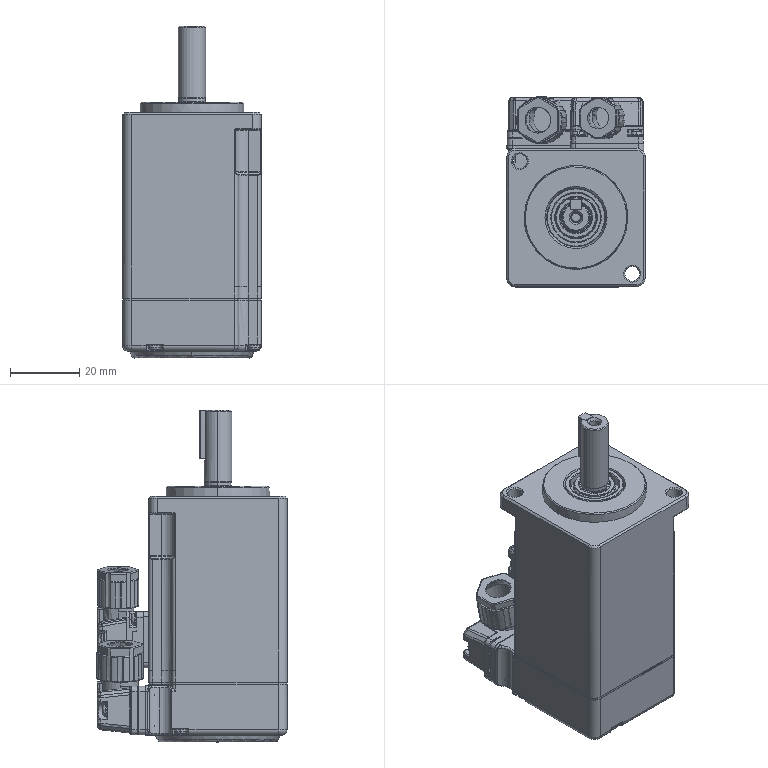Part | STEP file | X2MH010A-N2C (connector type) -1 | 1 solid | 2005 faces | box 40 x 54.95 x 96 mm | volume 118411 mm3 | spline 924 | plane 606 | cylinder 297 | torus 90 | cone 88 | commonest cylinder face diameters 3 x51 0.6 x44 0.4 x33 2.5 x23 3.3 x22 0.1 x16